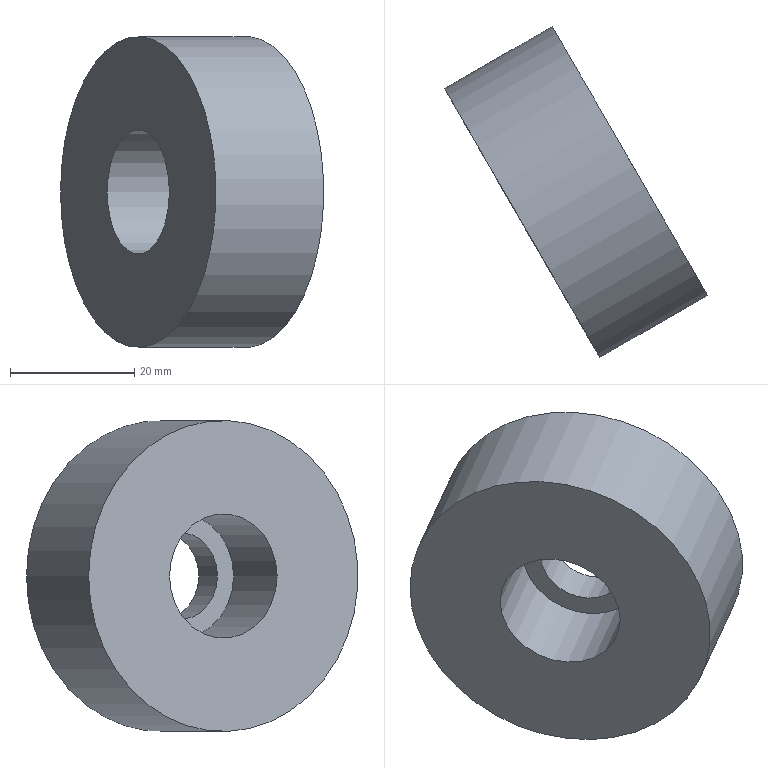Part | NX | features solid 2 | 1 solid | 6 faces | box 42.321 x 53.301 x 50 mm | volume 33948 mm3 | plane 3 | cylinder 3 | commonest cylinder face diameters 14 x1 20 x1 50 x1
STEP:
#1=CARTESIAN_POINT('',(-1278.041,-88.535,5.));
#2=VERTEX_POINT('',#1);
#3=CARTESIAN_POINT('',(-1273.041,-97.196,5.));
#4=DIRECTION('',(0.866,0.5,0.));
#5=DIRECTION('',(-0.5,0.866,0.));
#6=AXIS2_PLACEMENT_3D('',#3,#4,#5);
#7=CIRCLE('',#6,10.);
#8=EDGE_CURVE('',#2,#2,#7,.T.);
#9=ORIENTED_EDGE('',*,*,#8,.T.);
#10=EDGE_LOOP('',(#9));
#11=FACE_BOUND('',#10,.T.);
#12=CARTESIAN_POINT('',(-1285.541,-75.545,5.));
#13=VERTEX_POINT('',#12);
#14=CARTESIAN_POINT('',(-1273.041,-97.196,5.));
#15=DIRECTION('',(0.866,0.5,0.));
#16=DIRECTION('',(-0.5,0.866,0.));
#17=AXIS2_PLACEMENT_3D('',#14,#15,#16);
#18=CIRCLE('',#17,25.);
#19=EDGE_CURVE('',#13,#13,#18,.T.);
#20=ORIENTED_EDGE('',*,*,#19,.F.);
#21=EDGE_LOOP('',(#20));
#22=FACE_BOUND('',#21,.T.);
#23=CARTESIAN_POINT('',(-1273.041,-97.196,5.));
#24=DIRECTION('',(-0.866,-0.5,0.));
#25=DIRECTION('',(0.5,-0.866,0.));
#26=AXIS2_PLACEMENT_3D('',#23,#24,#25);
#27=PLANE('',#26);
#28=ADVANCED_FACE('',(#11,#22),#27,.T.);
#29=CARTESIAN_POINT('',(-1252.22,-93.258,5.));
#30=VERTEX_POINT('',#29);
#31=CARTESIAN_POINT('',(-1255.72,-87.196,5.));
#32=DIRECTION('',(-0.866,-0.5,0.));
#33=DIRECTION('',(0.5,-0.866,0.));
#34=AXIS2_PLACEMENT_3D('',#31,#32,#33);
#35=CIRCLE('',#34,7.);
#36=EDGE_CURVE('',#30,#30,#35,.T.);
#37=ORIENTED_EDGE('',*,*,#36,.T.);
#38=EDGE_LOOP('',(#37));
#39=FACE_BOUND('',#38,.T.);
#40=CARTESIAN_POINT('',(-1268.22,-65.545,5.));
#41=VERTEX_POINT('',#40);
#42=CARTESIAN_POINT('',(-1255.72,-87.196,5.));
#43=DIRECTION('',(0.866,0.5,0.));
#44=DIRECTION('',(-0.5,0.866,0.));
#45=AXIS2_PLACEMENT_3D('',#42,#43,#44);
#46=CIRCLE('',#45,25.);
#47=EDGE_CURVE('',#41,#41,#46,.T.);
#48=ORIENTED_EDGE('',*,*,#47,.T.);
#49=EDGE_LOOP('',(#48));
#50=FACE_BOUND('',#49,.T.);
#51=CARTESIAN_POINT('',(-1255.72,-87.196,5.));
#52=DIRECTION('',(-0.866,-0.5,0.));
#53=DIRECTION('',(0.5,-0.866,0.));
#54=AXIS2_PLACEMENT_3D('',#51,#52,#53);
#55=PLANE('',#54);
#56=ADVANCED_FACE('',(#39,#50),#55,.F.);
#57=ORIENTED_EDGE('',*,*,#19,.T.);
#58=EDGE_LOOP('',(#57));
#59=FACE_BOUND('',#58,.T.);
#60=ORIENTED_EDGE('',*,*,#47,.F.);
#61=EDGE_LOOP('',(#60));
#62=FACE_BOUND('',#61,.T.);
#63=CARTESIAN_POINT('',(-1255.72,-87.196,5.));
#64=DIRECTION('',(-0.866,-0.5,0.));
#65=DIRECTION('',(0.5,-0.866,0.));
#66=AXIS2_PLACEMENT_3D('',#63,#64,#65);
#67=CYLINDRICAL_SURFACE('',#66,25.);
#68=ADVANCED_FACE('',(#59,#62),#67,.T.);
#69=CARTESIAN_POINT('',(-1264.417,-84.134,5.));
#70=VERTEX_POINT('',#69);
#71=CARTESIAN_POINT('',(-1260.917,-90.196,5.));
#72=DIRECTION('',(0.866,0.5,0.));
#73=DIRECTION('',(-0.5,0.866,0.));
#74=AXIS2_PLACEMENT_3D('',#71,#72,#73);
#75=CIRCLE('',#74,7.);
#76=EDGE_CURVE('',#70,#70,#75,.T.);
#77=ORIENTED_EDGE('',*,*,#76,.F.);
#78=EDGE_LOOP('',(#77));
#79=FACE_BOUND('',#78,.T.);
#80=ORIENTED_EDGE('',*,*,#36,.F.);
#81=EDGE_LOOP('',(#80));
#82=FACE_BOUND('',#81,.T.);
#83=CARTESIAN_POINT('',(-1229.74,-72.196,5.));
#84=DIRECTION('',(0.866,0.5,0.));
#85=DIRECTION('',(-0.5,0.866,0.));
#86=AXIS2_PLACEMENT_3D('',#83,#84,#85);
#87=CYLINDRICAL_SURFACE('',#86,7.);
#88=ADVANCED_FACE('',(#79,#82),#87,.F.);
#89=ORIENTED_EDGE('',*,*,#76,.T.);
#90=EDGE_LOOP('',(#89));
#91=FACE_BOUND('',#90,.T.);
#92=CARTESIAN_POINT('',(-1265.917,-81.535,5.));
#93=VERTEX_POINT('',#92);
#94=CARTESIAN_POINT('',(-1260.917,-90.196,5.));
#95=DIRECTION('',(0.866,0.5,0.));
#96=DIRECTION('',(-0.5,0.866,0.));
#97=AXIS2_PLACEMENT_3D('',#94,#95,#96);
#98=CIRCLE('',#97,10.);
#99=EDGE_CURVE('',#93,#93,#98,.T.);
#100=ORIENTED_EDGE('',*,*,#99,.F.);
#101=EDGE_LOOP('',(#100));
#102=FACE_BOUND('',#101,.T.);
#103=CARTESIAN_POINT('',(-1260.917,-90.196,5.));
#104=DIRECTION('',(0.866,0.5,0.));
#105=DIRECTION('',(-0.5,0.866,0.));
#106=AXIS2_PLACEMENT_3D('',#103,#104,#105);
#107=PLANE('',#106);
#108=ADVANCED_FACE('',(#91,#102),#107,.F.);
#109=ORIENTED_EDGE('',*,*,#99,.T.);
#110=EDGE_LOOP('',(#109));
#111=FACE_BOUND('',#110,.T.);
#112=ORIENTED_EDGE('',*,*,#8,.F.);
#113=EDGE_LOOP('',(#112));
#114=FACE_BOUND('',#113,.T.);
#115=CARTESIAN_POINT('',(-1273.041,-97.196,5.));
#116=DIRECTION('',(0.866,0.5,0.));
#117=DIRECTION('',(-0.5,0.866,0.));
#118=AXIS2_PLACEMENT_3D('',#115,#116,#117);
#119=CYLINDRICAL_SURFACE('',#118,10.);
#120=ADVANCED_FACE('',(#111,#114),#119,.F.);
#121=CLOSED_SHELL('',(#28,#56,#68,#88,#108,#120));
#122=MANIFOLD_SOLID_BREP('',#121);
#123=(LENGTH_UNIT()NAMED_UNIT(*)SI_UNIT(.MILLI.,.METRE.));
#124=UNCERTAINTY_MEASURE_WITH_UNIT(LENGTH_MEASURE(0.00001),#123,'','');
#125=(NAMED_UNIT(*)PLANE_ANGLE_UNIT()SI_UNIT($,.RADIAN.));
#126=(NAMED_UNIT(*)SI_UNIT($,.STERADIAN.)SOLID_ANGLE_UNIT());
#127=(GEOMETRIC_REPRESENTATION_CONTEXT(3)GLOBAL_UNCERTAINTY_ASSIGNED_CONTEXT((#124))GLOBAL_UNIT_ASSIGNED_CONTEXT((#123,#125,#126))REPRESENTATION_CONTEXT('',''));
#128=ADVANCED_BREP_SHAPE_REPRESENTATION('',(#122),#127);